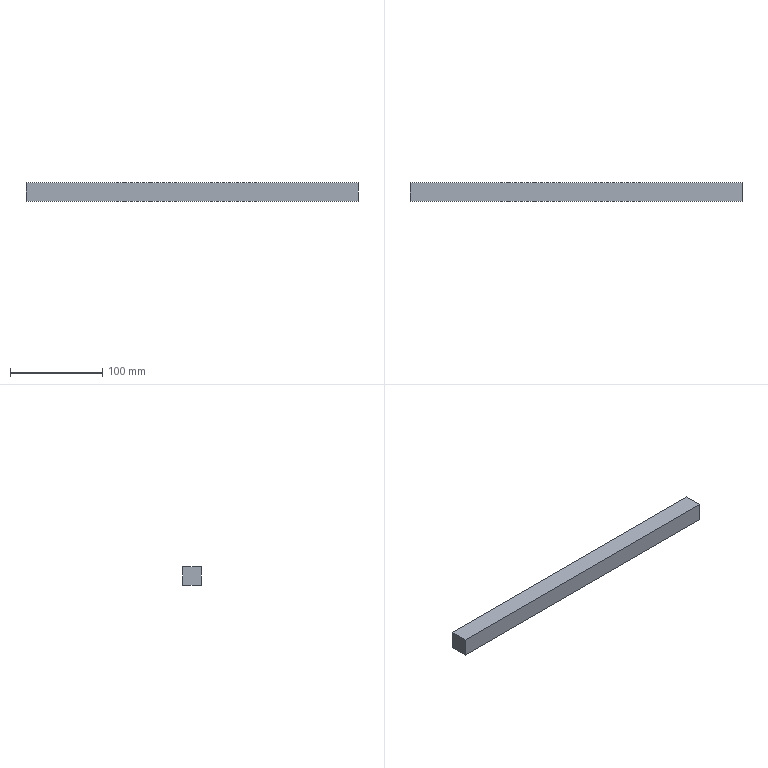Part | STEP file | 123_id954_x_t | 1 solid | 6 faces | box 360 x 20 x 20 mm | volume 144000 mm3 | plane 6
STEP:
#1=CARTESIAN_POINT('',(0.,0.,0.));
#2=DIRECTION('',(0.,0.,1.));
#3=DIRECTION('',(1.,0.,0.));
#4=AXIS2_PLACEMENT_3D('',#1,#2,#3);
#5=CARTESIAN_POINT('',(790.5,700.,150.));
#6=VERTEX_POINT('',#5);
#7=CARTESIAN_POINT('',(430.5,700.,150.));
#8=VERTEX_POINT('',#7);
#9=CARTESIAN_POINT('',(610.5,700.,150.));
#10=DIRECTION('',(-1.,0.,0.));
#11=VECTOR('',#10,1.);
#12=LINE('',#9,#11);
#13=CARTESIAN_POINT('',(610.5,710.,150.));
#14=DIRECTION('',(0.,0.,1.));
#15=DIRECTION('',(1.,0.,0.));
#16=AXIS2_PLACEMENT_3D('',#13,#14,#15);
#17=PLANE('',#16);
#18=CARTESIAN_POINT('',(0.,-10.));
#19=DIRECTION('',(-1.,0.));
#20=VECTOR('',#19,1.);
#21=LINE('',#18,#20);
#22=(GEOMETRIC_REPRESENTATION_CONTEXT(2)PARAMETRIC_REPRESENTATION_CONTEXT()REPRESENTATION_CONTEXT('',''));
#23=DEFINITIONAL_REPRESENTATION('',(#21),#22);
#24=PCURVE('',#17,#23);
#25=CARTESIAN_POINT('',(610.5,700.,130.));
#26=DIRECTION('',(0.,-1.,0.));
#27=DIRECTION('',(0.,0.,-1.));
#28=AXIS2_PLACEMENT_3D('',#25,#26,#27);
#29=PLANE('',#28);
#30=CARTESIAN_POINT('',(-20.,0.));
#31=DIRECTION('',(0.,-1.));
#32=VECTOR('',#31,1.);
#33=LINE('',#30,#32);
#34=(GEOMETRIC_REPRESENTATION_CONTEXT(2)PARAMETRIC_REPRESENTATION_CONTEXT()REPRESENTATION_CONTEXT('',''));
#35=DEFINITIONAL_REPRESENTATION('',(#33),#34);
#36=PCURVE('',#29,#35);
#37=SURFACE_CURVE('',#12,(#24,#36),.PCURVE_S1.);
#38=EDGE_CURVE('',#6,#8,#37,.T.);
#39=ORIENTED_EDGE('',*,*,#38,.F.);
#40=CARTESIAN_POINT('',(790.5,720.,150.));
#41=VERTEX_POINT('',#40);
#42=CARTESIAN_POINT('',(790.5,710.,150.));
#43=DIRECTION('',(0.,-1.,0.));
#44=VECTOR('',#43,1.);
#45=LINE('',#42,#44);
#46=CARTESIAN_POINT('',(180.,0.));
#47=DIRECTION('',(0.,-1.));
#48=VECTOR('',#47,1.);
#49=LINE('',#46,#48);
#50=(GEOMETRIC_REPRESENTATION_CONTEXT(2)PARAMETRIC_REPRESENTATION_CONTEXT()REPRESENTATION_CONTEXT('',''));
#51=DEFINITIONAL_REPRESENTATION('',(#49),#50);
#52=PCURVE('',#17,#51);
#53=CARTESIAN_POINT('',(790.5,710.,130.));
#54=DIRECTION('',(1.,0.,0.));
#55=DIRECTION('',(0.,0.,-1.));
#56=AXIS2_PLACEMENT_3D('',#53,#54,#55);
#57=PLANE('',#56);
#58=CARTESIAN_POINT('',(-20.,0.));
#59=DIRECTION('',(0.,-1.));
#60=VECTOR('',#59,1.);
#61=LINE('',#58,#60);
#62=(GEOMETRIC_REPRESENTATION_CONTEXT(2)PARAMETRIC_REPRESENTATION_CONTEXT()REPRESENTATION_CONTEXT('',''));
#63=DEFINITIONAL_REPRESENTATION('',(#61),#62);
#64=PCURVE('',#57,#63);
#65=SURFACE_CURVE('',#45,(#52,#64),.PCURVE_S1.);
#66=EDGE_CURVE('',#41,#6,#65,.T.);
#67=ORIENTED_EDGE('',*,*,#66,.F.);
#68=CARTESIAN_POINT('',(430.5,720.,150.));
#69=VERTEX_POINT('',#68);
#70=CARTESIAN_POINT('',(610.5,720.,150.));
#71=DIRECTION('',(1.,0.,0.));
#72=VECTOR('',#71,1.);
#73=LINE('',#70,#72);
#74=CARTESIAN_POINT('',(0.,10.));
#75=DIRECTION('',(1.,0.));
#76=VECTOR('',#75,1.);
#77=LINE('',#74,#76);
#78=(GEOMETRIC_REPRESENTATION_CONTEXT(2)PARAMETRIC_REPRESENTATION_CONTEXT()REPRESENTATION_CONTEXT('',''));
#79=DEFINITIONAL_REPRESENTATION('',(#77),#78);
#80=PCURVE('',#17,#79);
#81=CARTESIAN_POINT('',(610.5,720.,130.));
#82=DIRECTION('',(0.,1.,0.));
#83=DIRECTION('',(0.,0.,1.));
#84=AXIS2_PLACEMENT_3D('',#81,#82,#83);
#85=PLANE('',#84);
#86=CARTESIAN_POINT('',(20.,0.));
#87=DIRECTION('',(0.,1.));
#88=VECTOR('',#87,1.);
#89=LINE('',#86,#88);
#90=(GEOMETRIC_REPRESENTATION_CONTEXT(2)PARAMETRIC_REPRESENTATION_CONTEXT()REPRESENTATION_CONTEXT('',''));
#91=DEFINITIONAL_REPRESENTATION('',(#89),#90);
#92=PCURVE('',#85,#91);
#93=SURFACE_CURVE('',#73,(#80,#92),.PCURVE_S1.);
#94=EDGE_CURVE('',#69,#41,#93,.T.);
#95=ORIENTED_EDGE('',*,*,#94,.F.);
#96=CARTESIAN_POINT('',(430.5,710.,150.));
#97=DIRECTION('',(0.,1.,0.));
#98=VECTOR('',#97,1.);
#99=LINE('',#96,#98);
#100=CARTESIAN_POINT('',(-180.,0.));
#101=DIRECTION('',(0.,1.));
#102=VECTOR('',#101,1.);
#103=LINE('',#100,#102);
#104=(GEOMETRIC_REPRESENTATION_CONTEXT(2)PARAMETRIC_REPRESENTATION_CONTEXT()REPRESENTATION_CONTEXT('',''));
#105=DEFINITIONAL_REPRESENTATION('',(#103),#104);
#106=PCURVE('',#17,#105);
#107=CARTESIAN_POINT('',(430.5,710.,130.));
#108=DIRECTION('',(-1.,0.,0.));
#109=DIRECTION('',(0.,0.,1.));
#110=AXIS2_PLACEMENT_3D('',#107,#108,#109);
#111=PLANE('',#110);
#112=CARTESIAN_POINT('',(20.,0.));
#113=DIRECTION('',(0.,1.));
#114=VECTOR('',#113,1.);
#115=LINE('',#112,#114);
#116=(GEOMETRIC_REPRESENTATION_CONTEXT(2)PARAMETRIC_REPRESENTATION_CONTEXT()REPRESENTATION_CONTEXT('',''));
#117=DEFINITIONAL_REPRESENTATION('',(#115),#116);
#118=PCURVE('',#111,#117);
#119=SURFACE_CURVE('',#99,(#106,#118),.PCURVE_S1.);
#120=EDGE_CURVE('',#8,#69,#119,.T.);
#121=ORIENTED_EDGE('',*,*,#120,.F.);
#122=EDGE_LOOP('',(#39,#67,#95,#121));
#123=FACE_BOUND('',#122,.T.);
#124=ADVANCED_FACE('',(#123),#17,.T.);
#125=CARTESIAN_POINT('',(790.5,700.,130.));
#126=VERTEX_POINT('',#125);
#127=CARTESIAN_POINT('',(790.5,700.,130.));
#128=DIRECTION('',(0.,0.,1.));
#129=VECTOR('',#128,1.);
#130=LINE('',#127,#129);
#131=CARTESIAN_POINT('',(0.,180.));
#132=DIRECTION('',(-1.,0.));
#133=VECTOR('',#132,1.);
#134=LINE('',#131,#133);
#135=(GEOMETRIC_REPRESENTATION_CONTEXT(2)PARAMETRIC_REPRESENTATION_CONTEXT()REPRESENTATION_CONTEXT('',''));
#136=DEFINITIONAL_REPRESENTATION('',(#134),#135);
#137=PCURVE('',#29,#136);
#138=CARTESIAN_POINT('',(0.,-10.));
#139=DIRECTION('',(-1.,0.));
#140=VECTOR('',#139,1.);
#141=LINE('',#138,#140);
#142=(GEOMETRIC_REPRESENTATION_CONTEXT(2)PARAMETRIC_REPRESENTATION_CONTEXT()REPRESENTATION_CONTEXT('',''));
#143=DEFINITIONAL_REPRESENTATION('',(#141),#142);
#144=PCURVE('',#57,#143);
#145=SURFACE_CURVE('',#130,(#137,#144),.PCURVE_S1.);
#146=EDGE_CURVE('',#126,#6,#145,.T.);
#147=ORIENTED_EDGE('',*,*,#146,.T.);
#148=ORIENTED_EDGE('',*,*,#38,.T.);
#149=CARTESIAN_POINT('',(430.5,700.,130.));
#150=VERTEX_POINT('',#149);
#151=CARTESIAN_POINT('',(430.5,700.,130.));
#152=DIRECTION('',(0.,0.,1.));
#153=VECTOR('',#152,1.);
#154=LINE('',#151,#153);
#155=CARTESIAN_POINT('',(0.,-180.));
#156=DIRECTION('',(-1.,0.));
#157=VECTOR('',#156,1.);
#158=LINE('',#155,#157);
#159=(GEOMETRIC_REPRESENTATION_CONTEXT(2)PARAMETRIC_REPRESENTATION_CONTEXT()REPRESENTATION_CONTEXT('',''));
#160=DEFINITIONAL_REPRESENTATION('',(#158),#159);
#161=PCURVE('',#29,#160);
#162=CARTESIAN_POINT('',(0.,-10.));
#163=DIRECTION('',(1.,0.));
#164=VECTOR('',#163,1.);
#165=LINE('',#162,#164);
#166=(GEOMETRIC_REPRESENTATION_CONTEXT(2)PARAMETRIC_REPRESENTATION_CONTEXT()REPRESENTATION_CONTEXT('',''));
#167=DEFINITIONAL_REPRESENTATION('',(#165),#166);
#168=PCURVE('',#111,#167);
#169=SURFACE_CURVE('',#154,(#161,#168),.PCURVE_S1.);
#170=EDGE_CURVE('',#150,#8,#169,.T.);
#171=ORIENTED_EDGE('',*,*,#170,.F.);
#172=CARTESIAN_POINT('',(610.5,700.,130.));
#173=DIRECTION('',(1.,0.,0.));
#174=VECTOR('',#173,1.);
#175=LINE('',#172,#174);
#176=CARTESIAN_POINT('',(0.,0.));
#177=DIRECTION('',(0.,1.));
#178=VECTOR('',#177,1.);
#179=LINE('',#176,#178);
#180=(GEOMETRIC_REPRESENTATION_CONTEXT(2)PARAMETRIC_REPRESENTATION_CONTEXT()REPRESENTATION_CONTEXT('',''));
#181=DEFINITIONAL_REPRESENTATION('',(#179),#180);
#182=PCURVE('',#29,#181);
#183=CARTESIAN_POINT('',(610.5,710.,130.));
#184=DIRECTION('',(0.,0.,-1.));
#185=DIRECTION('',(-1.,0.,0.));
#186=AXIS2_PLACEMENT_3D('',#183,#184,#185);
#187=PLANE('',#186);
#188=CARTESIAN_POINT('',(0.,-10.));
#189=DIRECTION('',(-1.,0.));
#190=VECTOR('',#189,1.);
#191=LINE('',#188,#190);
#192=(GEOMETRIC_REPRESENTATION_CONTEXT(2)PARAMETRIC_REPRESENTATION_CONTEXT()REPRESENTATION_CONTEXT('',''));
#193=DEFINITIONAL_REPRESENTATION('',(#191),#192);
#194=PCURVE('',#187,#193);
#195=SURFACE_CURVE('',#175,(#182,#194),.PCURVE_S1.);
#196=EDGE_CURVE('',#150,#126,#195,.T.);
#197=ORIENTED_EDGE('',*,*,#196,.T.);
#198=EDGE_LOOP('',(#147,#148,#171,#197));
#199=FACE_BOUND('',#198,.T.);
#200=ADVANCED_FACE('',(#199),#29,.T.);
#201=ORIENTED_EDGE('',*,*,#170,.T.);
#202=ORIENTED_EDGE('',*,*,#120,.T.);
#203=CARTESIAN_POINT('',(430.5,720.,130.));
#204=VERTEX_POINT('',#203);
#205=CARTESIAN_POINT('',(430.5,720.,130.));
#206=DIRECTION('',(0.,0.,1.));
#207=VECTOR('',#206,1.);
#208=LINE('',#205,#207);
#209=CARTESIAN_POINT('',(0.,10.));
#210=DIRECTION('',(1.,0.));
#211=VECTOR('',#210,1.);
#212=LINE('',#209,#211);
#213=(GEOMETRIC_REPRESENTATION_CONTEXT(2)PARAMETRIC_REPRESENTATION_CONTEXT()REPRESENTATION_CONTEXT('',''));
#214=DEFINITIONAL_REPRESENTATION('',(#212),#213);
#215=PCURVE('',#111,#214);
#216=CARTESIAN_POINT('',(0.,-180.));
#217=DIRECTION('',(1.,0.));
#218=VECTOR('',#217,1.);
#219=LINE('',#216,#218);
#220=(GEOMETRIC_REPRESENTATION_CONTEXT(2)PARAMETRIC_REPRESENTATION_CONTEXT()REPRESENTATION_CONTEXT('',''));
#221=DEFINITIONAL_REPRESENTATION('',(#219),#220);
#222=PCURVE('',#85,#221);
#223=SURFACE_CURVE('',#208,(#215,#222),.PCURVE_S1.);
#224=EDGE_CURVE('',#204,#69,#223,.T.);
#225=ORIENTED_EDGE('',*,*,#224,.F.);
#226=CARTESIAN_POINT('',(430.5,710.,130.));
#227=DIRECTION('',(0.,-1.,0.));
#228=VECTOR('',#227,1.);
#229=LINE('',#226,#228);
#230=CARTESIAN_POINT('',(0.,0.));
#231=DIRECTION('',(0.,-1.));
#232=VECTOR('',#231,1.);
#233=LINE('',#230,#232);
#234=(GEOMETRIC_REPRESENTATION_CONTEXT(2)PARAMETRIC_REPRESENTATION_CONTEXT()REPRESENTATION_CONTEXT('',''));
#235=DEFINITIONAL_REPRESENTATION('',(#233),#234);
#236=PCURVE('',#111,#235);
#237=CARTESIAN_POINT('',(180.,0.));
#238=DIRECTION('',(0.,-1.));
#239=VECTOR('',#238,1.);
#240=LINE('',#237,#239);
#241=(GEOMETRIC_REPRESENTATION_CONTEXT(2)PARAMETRIC_REPRESENTATION_CONTEXT()REPRESENTATION_CONTEXT('',''));
#242=DEFINITIONAL_REPRESENTATION('',(#240),#241);
#243=PCURVE('',#187,#242);
#244=SURFACE_CURVE('',#229,(#236,#243),.PCURVE_S1.);
#245=EDGE_CURVE('',#204,#150,#244,.T.);
#246=ORIENTED_EDGE('',*,*,#245,.T.);
#247=EDGE_LOOP('',(#201,#202,#225,#246));
#248=FACE_BOUND('',#247,.T.);
#249=ADVANCED_FACE('',(#248),#111,.T.);
#250=ORIENTED_EDGE('',*,*,#224,.T.);
#251=ORIENTED_EDGE('',*,*,#94,.T.);
#252=CARTESIAN_POINT('',(790.5,720.,130.));
#253=VERTEX_POINT('',#252);
#254=CARTESIAN_POINT('',(790.5,720.,130.));
#255=DIRECTION('',(0.,0.,1.));
#256=VECTOR('',#255,1.);
#257=LINE('',#254,#256);
#258=CARTESIAN_POINT('',(0.,180.));
#259=DIRECTION('',(1.,0.));
#260=VECTOR('',#259,1.);
#261=LINE('',#258,#260);
#262=(GEOMETRIC_REPRESENTATION_CONTEXT(2)PARAMETRIC_REPRESENTATION_CONTEXT()REPRESENTATION_CONTEXT('',''));
#263=DEFINITIONAL_REPRESENTATION('',(#261),#262);
#264=PCURVE('',#85,#263);
#265=CARTESIAN_POINT('',(0.,10.));
#266=DIRECTION('',(-1.,0.));
#267=VECTOR('',#266,1.);
#268=LINE('',#265,#267);
#269=(GEOMETRIC_REPRESENTATION_CONTEXT(2)PARAMETRIC_REPRESENTATION_CONTEXT()REPRESENTATION_CONTEXT('',''));
#270=DEFINITIONAL_REPRESENTATION('',(#268),#269);
#271=PCURVE('',#57,#270);
#272=SURFACE_CURVE('',#257,(#264,#271),.PCURVE_S1.);
#273=EDGE_CURVE('',#253,#41,#272,.T.);
#274=ORIENTED_EDGE('',*,*,#273,.F.);
#275=CARTESIAN_POINT('',(610.5,720.,130.));
#276=DIRECTION('',(-1.,0.,0.));
#277=VECTOR('',#276,1.);
#278=LINE('',#275,#277);
#279=CARTESIAN_POINT('',(0.,0.));
#280=DIRECTION('',(0.,-1.));
#281=VECTOR('',#280,1.);
#282=LINE('',#279,#281);
#283=(GEOMETRIC_REPRESENTATION_CONTEXT(2)PARAMETRIC_REPRESENTATION_CONTEXT()REPRESENTATION_CONTEXT('',''));
#284=DEFINITIONAL_REPRESENTATION('',(#282),#283);
#285=PCURVE('',#85,#284);
#286=CARTESIAN_POINT('',(0.,10.));
#287=DIRECTION('',(1.,0.));
#288=VECTOR('',#287,1.);
#289=LINE('',#286,#288);
#290=(GEOMETRIC_REPRESENTATION_CONTEXT(2)PARAMETRIC_REPRESENTATION_CONTEXT()REPRESENTATION_CONTEXT('',''));
#291=DEFINITIONAL_REPRESENTATION('',(#289),#290);
#292=PCURVE('',#187,#291);
#293=SURFACE_CURVE('',#278,(#285,#292),.PCURVE_S1.);
#294=EDGE_CURVE('',#253,#204,#293,.T.);
#295=ORIENTED_EDGE('',*,*,#294,.T.);
#296=EDGE_LOOP('',(#250,#251,#274,#295));
#297=FACE_BOUND('',#296,.T.);
#298=ADVANCED_FACE('',(#297),#85,.T.);
#299=CARTESIAN_POINT('',(790.5,710.,130.));
#300=DIRECTION('',(0.,1.,0.));
#301=VECTOR('',#300,1.);
#302=LINE('',#299,#301);
#303=CARTESIAN_POINT('',(-180.,0.));
#304=DIRECTION('',(0.,1.));
#305=VECTOR('',#304,1.);
#306=LINE('',#303,#305);
#307=(GEOMETRIC_REPRESENTATION_CONTEXT(2)PARAMETRIC_REPRESENTATION_CONTEXT()REPRESENTATION_CONTEXT('',''));
#308=DEFINITIONAL_REPRESENTATION('',(#306),#307);
#309=PCURVE('',#187,#308);
#310=CARTESIAN_POINT('',(0.,0.));
#311=DIRECTION('',(0.,1.));
#312=VECTOR('',#311,1.);
#313=LINE('',#310,#312);
#314=(GEOMETRIC_REPRESENTATION_CONTEXT(2)PARAMETRIC_REPRESENTATION_CONTEXT()REPRESENTATION_CONTEXT('',''));
#315=DEFINITIONAL_REPRESENTATION('',(#313),#314);
#316=PCURVE('',#57,#315);
#317=SURFACE_CURVE('',#302,(#309,#316),.PCURVE_S1.);
#318=EDGE_CURVE('',#126,#253,#317,.T.);
#319=ORIENTED_EDGE('',*,*,#318,.F.);
#320=ORIENTED_EDGE('',*,*,#196,.F.);
#321=ORIENTED_EDGE('',*,*,#245,.F.);
#322=ORIENTED_EDGE('',*,*,#294,.F.);
#323=EDGE_LOOP('',(#319,#320,#321,#322));
#324=FACE_BOUND('',#323,.T.);
#325=ADVANCED_FACE('',(#324),#187,.T.);
#326=ORIENTED_EDGE('',*,*,#318,.T.);
#327=ORIENTED_EDGE('',*,*,#273,.T.);
#328=ORIENTED_EDGE('',*,*,#66,.T.);
#329=ORIENTED_EDGE('',*,*,#146,.F.);
#330=EDGE_LOOP('',(#326,#327,#328,#329));
#331=FACE_BOUND('',#330,.T.);
#332=ADVANCED_FACE('',(#331),#57,.T.);
#333=CLOSED_SHELL('',(#124,#200,#249,#298,#325,#332));
#334=MANIFOLD_SOLID_BREP('',#333);
#335=(LENGTH_UNIT()NAMED_UNIT(*)SI_UNIT(.MILLI.,.METRE.));
#336=UNCERTAINTY_MEASURE_WITH_UNIT(LENGTH_MEASURE(0.0000001),#335,'','');
#337=(NAMED_UNIT(*)PLANE_ANGLE_UNIT()SI_UNIT($,.RADIAN.));
#338=(NAMED_UNIT(*)SI_UNIT($,.STERADIAN.)SOLID_ANGLE_UNIT());
#339=(GEOMETRIC_REPRESENTATION_CONTEXT(3)GLOBAL_UNCERTAINTY_ASSIGNED_CONTEXT((#336))GLOBAL_UNIT_ASSIGNED_CONTEXT((#335,#337,#338))REPRESENTATION_CONTEXT('',''));
#340=ADVANCED_BREP_SHAPE_REPRESENTATION('',(#4,#334),#339);